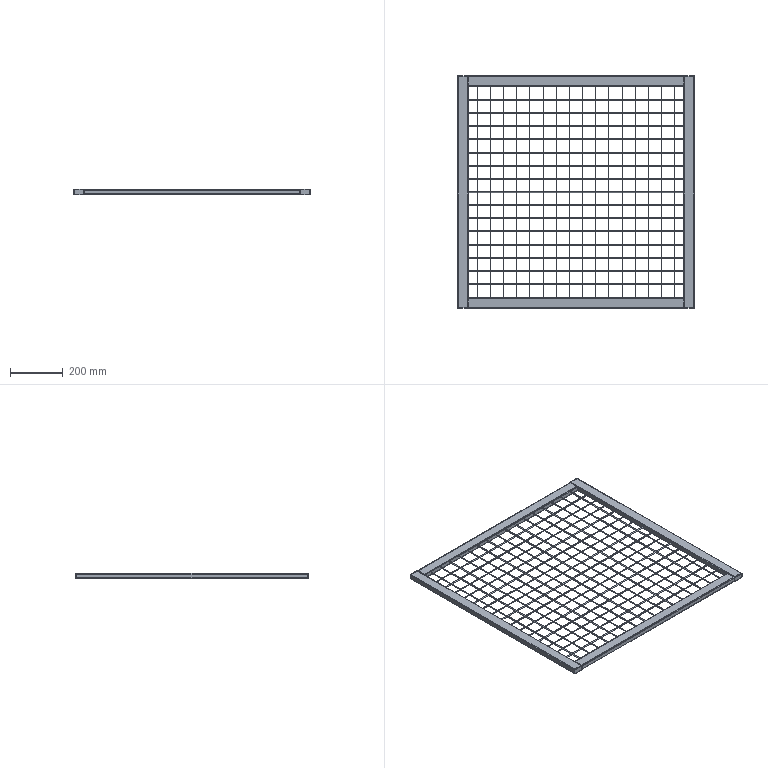Part | SolidWorks | features BaseBody 39 | 39 solids | 248 faces | box 900 x 885 x 20 mm | volume 1062813 mm3 | plane 126 | cylinder 122 | commonest cylinder face diameters 4 x62 6 x32 2 x16 6.8 x8 5 x4